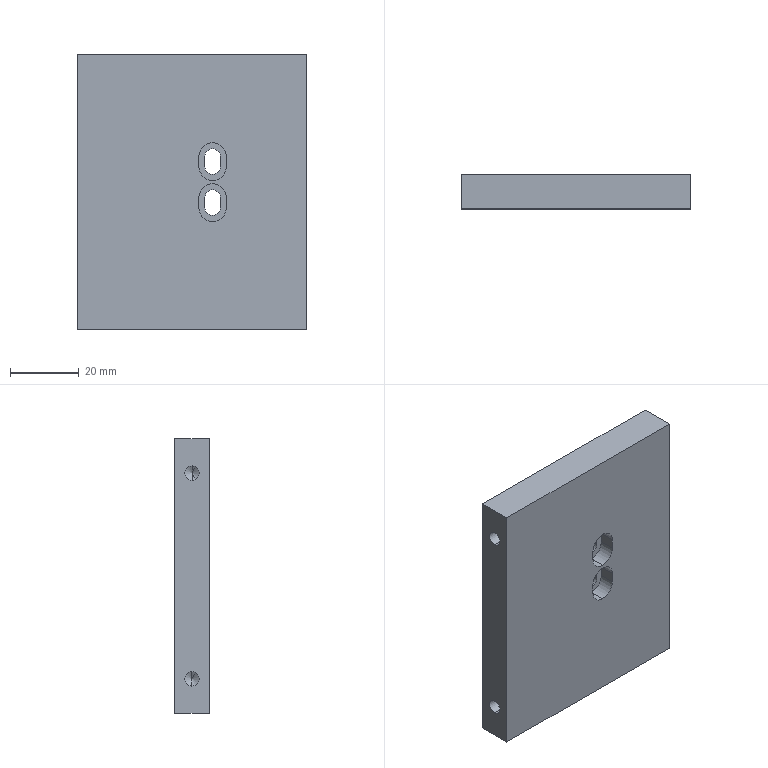Part | SolidWorks | features HoleWzd 2, Extrusion 1, MirrorPattern 1 | 1 solid | 44 faces | box 67 x 10 x 80 mm | volume 51889 mm3 | cylinder 20 | plane 16 | cone 8 | commonest cylinder face diameters 4.2 x8 4.5 x6 8 x6
STEP:
#1=CARTESIAN_POINT('',(6.,-0.4,3.376));
#2=VERTEX_POINT('',#1);
#3=CARTESIAN_POINT('',(10.,-0.4,7.376));
#4=VERTEX_POINT('',#3);
#5=CARTESIAN_POINT('',(6.,-0.4,7.376));
#6=DIRECTION('',(0.,-1.,0.));
#7=DIRECTION('',(0.,0.,-1.));
#8=AXIS2_PLACEMENT_3D('',#5,#6,#7);
#9=CIRCLE('',#8,4.);
#10=EDGE_CURVE('',#2,#4,#9,.T.);
#11=ORIENTED_EDGE('',*,*,#10,.F.);
#12=CARTESIAN_POINT('',(6.,-5.,3.376));
#13=VERTEX_POINT('',#12);
#14=CARTESIAN_POINT('',(6.,-5.,3.376));
#15=DIRECTION('',(0.,-1.,0.));
#16=VECTOR('',#15,1000.);
#17=LINE('',#14,#16);
#18=EDGE_CURVE('',#2,#13,#17,.T.);
#19=ORIENTED_EDGE('',*,*,#18,.T.);
#20=CARTESIAN_POINT('',(10.,-5.,7.376));
#21=VERTEX_POINT('',#20);
#22=CARTESIAN_POINT('',(6.,-5.,7.376));
#23=DIRECTION('',(0.,-1.,0.));
#24=DIRECTION('',(0.,0.,-1.));
#25=AXIS2_PLACEMENT_3D('',#22,#23,#24);
#26=CIRCLE('',#25,4.);
#27=EDGE_CURVE('',#13,#21,#26,.T.);
#28=ORIENTED_EDGE('',*,*,#27,.T.);
#29=CARTESIAN_POINT('',(10.,-0.4,7.376));
#30=DIRECTION('',(0.,1.,0.));
#31=VECTOR('',#30,1000.);
#32=LINE('',#29,#31);
#33=EDGE_CURVE('',#21,#4,#32,.T.);
#34=ORIENTED_EDGE('',*,*,#33,.T.);
#35=EDGE_LOOP('',(#11,#19,#28,#34));
#36=FACE_OUTER_BOUND('',#35,.T.);
#37=CARTESIAN_POINT('',(6.,-5.,7.376));
#38=DIRECTION('',(0.,-1.,0.));
#39=DIRECTION('',(0.,0.,-1.));
#40=AXIS2_PLACEMENT_3D('',#37,#38,#39);
#41=CYLINDRICAL_SURFACE('',#40,4.);
#42=ADVANCED_FACE('',(#36),#41,.F.);
#43=CARTESIAN_POINT('',(6.,5.,5.126));
#44=VERTEX_POINT('',#43);
#45=CARTESIAN_POINT('',(8.25,5.,7.376));
#46=VERTEX_POINT('',#45);
#47=CARTESIAN_POINT('',(6.,5.,7.376));
#48=DIRECTION('',(0.,-1.,0.));
#49=DIRECTION('',(0.,0.,-1.));
#50=AXIS2_PLACEMENT_3D('',#47,#48,#49);
#51=CIRCLE('',#50,2.25);
#52=EDGE_CURVE('',#44,#46,#51,.T.);
#53=ORIENTED_EDGE('',*,*,#52,.F.);
#54=CARTESIAN_POINT('',(6.,-0.4,5.126));
#55=VERTEX_POINT('',#54);
#56=CARTESIAN_POINT('',(6.,-5.,5.126));
#57=DIRECTION('',(0.,-1.,0.));
#58=VECTOR('',#57,1000.);
#59=LINE('',#56,#58);
#60=EDGE_CURVE('',#44,#55,#59,.T.);
#61=ORIENTED_EDGE('',*,*,#60,.T.);
#62=CARTESIAN_POINT('',(8.25,-0.4,7.376));
#63=VERTEX_POINT('',#62);
#64=CARTESIAN_POINT('',(6.,-0.4,7.376));
#65=DIRECTION('',(0.,-1.,0.));
#66=DIRECTION('',(0.,0.,-1.));
#67=AXIS2_PLACEMENT_3D('',#64,#65,#66);
#68=CIRCLE('',#67,2.25);
#69=EDGE_CURVE('',#55,#63,#68,.T.);
#70=ORIENTED_EDGE('',*,*,#69,.T.);
#71=CARTESIAN_POINT('',(8.25,5.,7.376));
#72=DIRECTION('',(0.,1.,0.));
#73=VECTOR('',#72,1000.);
#74=LINE('',#71,#73);
#75=EDGE_CURVE('',#63,#46,#74,.T.);
#76=ORIENTED_EDGE('',*,*,#75,.T.);
#77=EDGE_LOOP('',(#53,#61,#70,#76));
#78=FACE_OUTER_BOUND('',#77,.T.);
#79=CARTESIAN_POINT('',(6.,-5.,7.376));
#80=DIRECTION('',(0.,-1.,0.));
#81=DIRECTION('',(0.,0.,-1.));
#82=AXIS2_PLACEMENT_3D('',#79,#80,#81);
#83=CYLINDRICAL_SURFACE('',#82,2.25);
#84=ADVANCED_FACE('',(#78),#83,.F.);
#85=CARTESIAN_POINT('',(6.,-0.4,-8.624));
#86=VERTEX_POINT('',#85);
#87=CARTESIAN_POINT('',(10.,-0.4,-4.624));
#88=VERTEX_POINT('',#87);
#89=CARTESIAN_POINT('',(6.,-0.4,-4.624));
#90=DIRECTION('',(0.,-1.,0.));
#91=DIRECTION('',(0.,0.,-1.));
#92=AXIS2_PLACEMENT_3D('',#89,#90,#91);
#93=CIRCLE('',#92,4.);
#94=EDGE_CURVE('',#86,#88,#93,.T.);
#95=ORIENTED_EDGE('',*,*,#94,.F.);
#96=CARTESIAN_POINT('',(6.,-5.,-8.624));
#97=VERTEX_POINT('',#96);
#98=CARTESIAN_POINT('',(6.,-5.,-8.624));
#99=DIRECTION('',(0.,-1.,0.));
#100=VECTOR('',#99,1000.);
#101=LINE('',#98,#100);
#102=EDGE_CURVE('',#86,#97,#101,.T.);
#103=ORIENTED_EDGE('',*,*,#102,.T.);
#104=CARTESIAN_POINT('',(10.,-5.,-4.624));
#105=VERTEX_POINT('',#104);
#106=CARTESIAN_POINT('',(6.,-5.,-4.624));
#107=DIRECTION('',(0.,-1.,0.));
#108=DIRECTION('',(0.,0.,-1.));
#109=AXIS2_PLACEMENT_3D('',#106,#107,#108);
#110=CIRCLE('',#109,4.);
#111=EDGE_CURVE('',#97,#105,#110,.T.);
#112=ORIENTED_EDGE('',*,*,#111,.T.);
#113=CARTESIAN_POINT('',(10.,-0.4,-4.624));
#114=DIRECTION('',(0.,1.,0.));
#115=VECTOR('',#114,1000.);
#116=LINE('',#113,#115);
#117=EDGE_CURVE('',#105,#88,#116,.T.);
#118=ORIENTED_EDGE('',*,*,#117,.T.);
#119=EDGE_LOOP('',(#95,#103,#112,#118));
#120=FACE_OUTER_BOUND('',#119,.T.);
#121=CARTESIAN_POINT('',(6.,-5.,-4.624));
#122=DIRECTION('',(0.,-1.,0.));
#123=DIRECTION('',(0.,0.,-1.));
#124=AXIS2_PLACEMENT_3D('',#121,#122,#123);
#125=CYLINDRICAL_SURFACE('',#124,4.);
#126=ADVANCED_FACE('',(#120),#125,.F.);
#127=CARTESIAN_POINT('',(6.,5.,-6.874));
#128=VERTEX_POINT('',#127);
#129=CARTESIAN_POINT('',(8.25,5.,-4.624));
#130=VERTEX_POINT('',#129);
#131=CARTESIAN_POINT('',(6.,5.,-4.624));
#132=DIRECTION('',(0.,-1.,0.));
#133=DIRECTION('',(0.,0.,-1.));
#134=AXIS2_PLACEMENT_3D('',#131,#132,#133);
#135=CIRCLE('',#134,2.25);
#136=EDGE_CURVE('',#128,#130,#135,.T.);
#137=ORIENTED_EDGE('',*,*,#136,.F.);
#138=CARTESIAN_POINT('',(6.,-0.4,-6.874));
#139=VERTEX_POINT('',#138);
#140=CARTESIAN_POINT('',(6.,-5.,-6.874));
#141=DIRECTION('',(0.,-1.,0.));
#142=VECTOR('',#141,1000.);
#143=LINE('',#140,#142);
#144=EDGE_CURVE('',#128,#139,#143,.T.);
#145=ORIENTED_EDGE('',*,*,#144,.T.);
#146=CARTESIAN_POINT('',(8.25,-0.4,-4.624));
#147=VERTEX_POINT('',#146);
#148=CARTESIAN_POINT('',(6.,-0.4,-4.624));
#149=DIRECTION('',(0.,-1.,0.));
#150=DIRECTION('',(0.,0.,-1.));
#151=AXIS2_PLACEMENT_3D('',#148,#149,#150);
#152=CIRCLE('',#151,2.25);
#153=EDGE_CURVE('',#139,#147,#152,.T.);
#154=ORIENTED_EDGE('',*,*,#153,.T.);
#155=CARTESIAN_POINT('',(8.25,5.,-4.624));
#156=DIRECTION('',(0.,1.,0.));
#157=VECTOR('',#156,1000.);
#158=LINE('',#155,#157);
#159=EDGE_CURVE('',#147,#130,#158,.T.);
#160=ORIENTED_EDGE('',*,*,#159,.T.);
#161=EDGE_LOOP('',(#137,#145,#154,#160));
#162=FACE_OUTER_BOUND('',#161,.T.);
#163=CARTESIAN_POINT('',(6.,-5.,-4.624));
#164=DIRECTION('',(0.,-1.,0.));
#165=DIRECTION('',(0.,0.,-1.));
#166=AXIS2_PLACEMENT_3D('',#163,#164,#165);
#167=CYLINDRICAL_SURFACE('',#166,2.25);
#168=ADVANCED_FACE('',(#162),#167,.F.);
#169=CARTESIAN_POINT('',(-21.1,0.,27.9));
#170=VERTEX_POINT('',#169);
#171=CARTESIAN_POINT('',(-21.1,0.,32.1));
#172=VERTEX_POINT('',#171);
#173=CARTESIAN_POINT('',(-21.1,0.,30.));
#174=DIRECTION('',(-1.,0.,0.));
#175=DIRECTION('',(0.,0.,1.));
#176=AXIS2_PLACEMENT_3D('',#173,#174,#175);
#177=CIRCLE('',#176,2.1);
#178=EDGE_CURVE('',#170,#172,#177,.T.);
#179=ORIENTED_EDGE('',*,*,#178,.F.);
#180=CARTESIAN_POINT('',(-33.5,0.,27.9));
#181=VERTEX_POINT('',#180);
#182=CARTESIAN_POINT('',(-33.5,0.,27.9));
#183=DIRECTION('',(-1.,0.,0.));
#184=VECTOR('',#183,1000.);
#185=LINE('',#182,#184);
#186=EDGE_CURVE('',#170,#181,#185,.T.);
#187=ORIENTED_EDGE('',*,*,#186,.T.);
#188=CARTESIAN_POINT('',(-33.5,0.,32.1));
#189=VERTEX_POINT('',#188);
#190=CARTESIAN_POINT('',(-33.5,0.,30.));
#191=DIRECTION('',(-1.,0.,0.));
#192=DIRECTION('',(0.,0.,1.));
#193=AXIS2_PLACEMENT_3D('',#190,#191,#192);
#194=CIRCLE('',#193,2.1);
#195=EDGE_CURVE('',#181,#189,#194,.T.);
#196=ORIENTED_EDGE('',*,*,#195,.T.);
#197=CARTESIAN_POINT('',(-33.5,0.,32.1));
#198=DIRECTION('',(-1.,0.,0.));
#199=VECTOR('',#198,1000.);
#200=LINE('',#197,#199);
#201=EDGE_CURVE('',#172,#189,#200,.T.);
#202=ORIENTED_EDGE('',*,*,#201,.F.);
#203=EDGE_LOOP('',(#179,#187,#196,#202));
#204=FACE_OUTER_BOUND('',#203,.T.);
#205=CARTESIAN_POINT('',(-33.5,0.,30.));
#206=DIRECTION('',(-1.,0.,0.));
#207=DIRECTION('',(0.,0.,1.));
#208=AXIS2_PLACEMENT_3D('',#205,#206,#207);
#209=CYLINDRICAL_SURFACE('',#208,2.1);
#210=ADVANCED_FACE('',(#204),#209,.F.);
#211=CARTESIAN_POINT('',(-19.838,0.,30.));
#212=VERTEX_POINT('',#211);
#213=CARTESIAN_POINT('',(-21.1,0.,32.1));
#214=DIRECTION('',(-0.515,0.,0.8572));
#215=VECTOR('',#214,1000.);
#216=LINE('',#213,#215);
#217=EDGE_CURVE('',#212,#172,#216,.T.);
#218=ORIENTED_EDGE('',*,*,#217,.F.);
#219=CARTESIAN_POINT('',(-21.1,0.,27.9));
#220=DIRECTION('',(-0.515,0.,-0.8572));
#221=VECTOR('',#220,1000.);
#222=LINE('',#219,#221);
#223=EDGE_CURVE('',#212,#170,#222,.T.);
#224=ORIENTED_EDGE('',*,*,#223,.T.);
#225=ORIENTED_EDGE('',*,*,#178,.T.);
#226=EDGE_LOOP('',(#218,#224,#225));
#227=FACE_OUTER_BOUND('',#226,.T.);
#228=CARTESIAN_POINT('',(-21.1,0.,30.));
#229=DIRECTION('',(-1.,0.,0.));
#230=DIRECTION('',(0.,0.,1.));
#231=AXIS2_PLACEMENT_3D('',#228,#229,#230);
#232=CONICAL_SURFACE('',#231,2.1,1.03);
#233=ADVANCED_FACE('',(#227),#232,.F.);
#234=CARTESIAN_POINT('',(-21.1,0.,-32.1));
#235=VERTEX_POINT('',#234);
#236=CARTESIAN_POINT('',(-21.1,0.,-27.9));
#237=VERTEX_POINT('',#236);
#238=CARTESIAN_POINT('',(-21.1,0.,-30.));
#239=DIRECTION('',(-1.,0.,0.));
#240=DIRECTION('',(0.,0.,1.));
#241=AXIS2_PLACEMENT_3D('',#238,#239,#240);
#242=CIRCLE('',#241,2.1);
#243=EDGE_CURVE('',#235,#237,#242,.T.);
#244=ORIENTED_EDGE('',*,*,#243,.F.);
#245=CARTESIAN_POINT('',(-33.5,0.,-32.1));
#246=VERTEX_POINT('',#245);
#247=CARTESIAN_POINT('',(-33.5,0.,-32.1));
#248=DIRECTION('',(-1.,0.,0.));
#249=VECTOR('',#248,1000.);
#250=LINE('',#247,#249);
#251=EDGE_CURVE('',#235,#246,#250,.T.);
#252=ORIENTED_EDGE('',*,*,#251,.T.);
#253=CARTESIAN_POINT('',(-33.5,0.,-27.9));
#254=VERTEX_POINT('',#253);
#255=CARTESIAN_POINT('',(-33.5,0.,-30.));
#256=DIRECTION('',(-1.,0.,0.));
#257=DIRECTION('',(0.,0.,1.));
#258=AXIS2_PLACEMENT_3D('',#255,#256,#257);
#259=CIRCLE('',#258,2.1);
#260=EDGE_CURVE('',#246,#254,#259,.T.);
#261=ORIENTED_EDGE('',*,*,#260,.T.);
#262=CARTESIAN_POINT('',(-33.5,0.,-27.9));
#263=DIRECTION('',(-1.,0.,0.));
#264=VECTOR('',#263,1000.);
#265=LINE('',#262,#264);
#266=EDGE_CURVE('',#237,#254,#265,.T.);
#267=ORIENTED_EDGE('',*,*,#266,.F.);
#268=EDGE_LOOP('',(#244,#252,#261,#267));
#269=FACE_OUTER_BOUND('',#268,.T.);
#270=CARTESIAN_POINT('',(-33.5,0.,-30.));
#271=DIRECTION('',(-1.,0.,0.));
#272=DIRECTION('',(0.,0.,1.));
#273=AXIS2_PLACEMENT_3D('',#270,#271,#272);
#274=CYLINDRICAL_SURFACE('',#273,2.1);
#275=ADVANCED_FACE('',(#269),#274,.F.);
#276=CARTESIAN_POINT('',(-19.838,0.,-30.));
#277=VERTEX_POINT('',#276);
#278=CARTESIAN_POINT('',(-21.1,0.,-27.9));
#279=DIRECTION('',(-0.515,0.,0.8572));
#280=VECTOR('',#279,1000.);
#281=LINE('',#278,#280);
#282=EDGE_CURVE('',#277,#237,#281,.T.);
#283=ORIENTED_EDGE('',*,*,#282,.F.);
#284=CARTESIAN_POINT('',(-21.1,0.,-32.1));
#285=DIRECTION('',(-0.515,0.,-0.8572));
#286=VECTOR('',#285,1000.);
#287=LINE('',#284,#286);
#288=EDGE_CURVE('',#277,#235,#287,.T.);
#289=ORIENTED_EDGE('',*,*,#288,.T.);
#290=ORIENTED_EDGE('',*,*,#243,.T.);
#291=EDGE_LOOP('',(#283,#289,#290));
#292=FACE_OUTER_BOUND('',#291,.T.);
#293=CARTESIAN_POINT('',(-21.1,0.,-30.));
#294=DIRECTION('',(-1.,0.,0.));
#295=DIRECTION('',(0.,0.,1.));
#296=AXIS2_PLACEMENT_3D('',#293,#294,#295);
#297=CONICAL_SURFACE('',#296,2.1,1.03);
#298=ADVANCED_FACE('',(#292),#297,.F.);
#299=CARTESIAN_POINT('',(21.1,0.,32.1));
#300=VERTEX_POINT('',#299);
#301=CARTESIAN_POINT('',(21.1,0.,27.9));
#302=VERTEX_POINT('',#301);
#303=CARTESIAN_POINT('',(21.1,0.,30.));
#304=DIRECTION('',(1.,0.,0.));
#305=DIRECTION('',(0.,0.,-1.));
#306=AXIS2_PLACEMENT_3D('',#303,#304,#305);
#307=CIRCLE('',#306,2.1);
#308=EDGE_CURVE('',#300,#302,#307,.T.);
#309=ORIENTED_EDGE('',*,*,#308,.F.);
#310=CARTESIAN_POINT('',(33.5,0.,32.1));
#311=VERTEX_POINT('',#310);
#312=CARTESIAN_POINT('',(33.5,0.,32.1));
#313=DIRECTION('',(1.,0.,0.));
#314=VECTOR('',#313,1000.);
#315=LINE('',#312,#314);
#316=EDGE_CURVE('',#300,#311,#315,.T.);
#317=ORIENTED_EDGE('',*,*,#316,.T.);
#318=CARTESIAN_POINT('',(33.5,0.,27.9));
#319=VERTEX_POINT('',#318);
#320=CARTESIAN_POINT('',(33.5,0.,30.));
#321=DIRECTION('',(1.,0.,0.));
#322=DIRECTION('',(0.,0.,-1.));
#323=AXIS2_PLACEMENT_3D('',#320,#321,#322);
#324=CIRCLE('',#323,2.1);
#325=EDGE_CURVE('',#311,#319,#324,.T.);
#326=ORIENTED_EDGE('',*,*,#325,.T.);
#327=CARTESIAN_POINT('',(33.5,0.,27.9));
#328=DIRECTION('',(1.,0.,0.));
#329=VECTOR('',#328,1000.);
#330=LINE('',#327,#329);
#331=EDGE_CURVE('',#302,#319,#330,.T.);
#332=ORIENTED_EDGE('',*,*,#331,.F.);
#333=EDGE_LOOP('',(#309,#317,#326,#332));
#334=FACE_OUTER_BOUND('',#333,.T.);
#335=CARTESIAN_POINT('',(33.5,0.,30.));
#336=DIRECTION('',(1.,0.,0.));
#337=DIRECTION('',(0.,0.,-1.));
#338=AXIS2_PLACEMENT_3D('',#335,#336,#337);
#339=CYLINDRICAL_SURFACE('',#338,2.1);
#340=ADVANCED_FACE('',(#334),#339,.F.);
#341=CARTESIAN_POINT('',(19.838,0.,30.));
#342=VERTEX_POINT('',#341);
#343=CARTESIAN_POINT('',(21.1,0.,27.9));
#344=DIRECTION('',(0.515,0.,-0.8572));
#345=VECTOR('',#344,1000.);
#346=LINE('',#343,#345);
#347=EDGE_CURVE('',#342,#302,#346,.T.);
#348=ORIENTED_EDGE('',*,*,#347,.F.);
#349=CARTESIAN_POINT('',(21.1,0.,32.1));
#350=DIRECTION('',(0.515,0.,0.8572));
#351=VECTOR('',#350,1000.);
#352=LINE('',#349,#351);
#353=EDGE_CURVE('',#342,#300,#352,.T.);
#354=ORIENTED_EDGE('',*,*,#353,.T.);
#355=ORIENTED_EDGE('',*,*,#308,.T.);
#356=EDGE_LOOP('',(#348,#354,#355));
#357=FACE_OUTER_BOUND('',#356,.T.);
#358=CARTESIAN_POINT('',(21.1,0.,30.));
#359=DIRECTION('',(1.,0.,0.));
#360=DIRECTION('',(0.,0.,-1.));
#361=AXIS2_PLACEMENT_3D('',#358,#359,#360);
#362=CONICAL_SURFACE('',#361,2.1,1.03);
#363=ADVANCED_FACE('',(#357),#362,.F.);
#364=CARTESIAN_POINT('',(21.1,0.,-27.9));
#365=VERTEX_POINT('',#364);
#366=CARTESIAN_POINT('',(21.1,0.,-32.1));
#367=VERTEX_POINT('',#366);
#368=CARTESIAN_POINT('',(21.1,0.,-30.));
#369=DIRECTION('',(1.,0.,0.));
#370=DIRECTION('',(0.,0.,-1.));
#371=AXIS2_PLACEMENT_3D('',#368,#369,#370);
#372=CIRCLE('',#371,2.1);
#373=EDGE_CURVE('',#365,#367,#372,.T.);
#374=ORIENTED_EDGE('',*,*,#373,.F.);
#375=CARTESIAN_POINT('',(33.5,0.,-27.9));
#376=VERTEX_POINT('',#375);
#377=CARTESIAN_POINT('',(33.5,0.,-27.9));
#378=DIRECTION('',(1.,0.,0.));
#379=VECTOR('',#378,1000.);
#380=LINE('',#377,#379);
#381=EDGE_CURVE('',#365,#376,#380,.T.);
#382=ORIENTED_EDGE('',*,*,#381,.T.);
#383=CARTESIAN_POINT('',(33.5,0.,-32.1));
#384=VERTEX_POINT('',#383);
#385=CARTESIAN_POINT('',(33.5,0.,-30.));
#386=DIRECTION('',(1.,0.,0.));
#387=DIRECTION('',(0.,0.,-1.));
#388=AXIS2_PLACEMENT_3D('',#385,#386,#387);
#389=CIRCLE('',#388,2.1);
#390=EDGE_CURVE('',#376,#384,#389,.T.);
#391=ORIENTED_EDGE('',*,*,#390,.T.);
#392=CARTESIAN_POINT('',(33.5,0.,-32.1));
#393=DIRECTION('',(1.,0.,0.));
#394=VECTOR('',#393,1000.);
#395=LINE('',#392,#394);
#396=EDGE_CURVE('',#367,#384,#395,.T.);
#397=ORIENTED_EDGE('',*,*,#396,.F.);
#398=EDGE_LOOP('',(#374,#382,#391,#397));
#399=FACE_OUTER_BOUND('',#398,.T.);
#400=CARTESIAN_POINT('',(33.5,0.,-30.));
#401=DIRECTION('',(1.,0.,0.));
#402=DIRECTION('',(0.,0.,-1.));
#403=AXIS2_PLACEMENT_3D('',#400,#401,#402);
#404=CYLINDRICAL_SURFACE('',#403,2.1);
#405=ADVANCED_FACE('',(#399),#404,.F.);
#406=CARTESIAN_POINT('',(19.838,0.,-30.));
#407=VERTEX_POINT('',#406);
#408=CARTESIAN_POINT('',(21.1,0.,-32.1));
#409=DIRECTION('',(0.515,0.,-0.8572));
#410=VECTOR('',#409,1000.);
#411=LINE('',#408,#410);
#412=EDGE_CURVE('',#407,#367,#411,.T.);
#413=ORIENTED_EDGE('',*,*,#412,.F.);
#414=CARTESIAN_POINT('',(21.1,0.,-27.9));
#415=DIRECTION('',(0.515,0.,0.8572));
#416=VECTOR('',#415,1000.);
#417=LINE('',#414,#416);
#418=EDGE_CURVE('',#407,#365,#417,.T.);
#419=ORIENTED_EDGE('',*,*,#418,.T.);
#420=ORIENTED_EDGE('',*,*,#373,.T.);
#421=EDGE_LOOP('',(#413,#419,#420));
#422=FACE_OUTER_BOUND('',#421,.T.);
#423=CARTESIAN_POINT('',(21.1,0.,-30.));
#424=DIRECTION('',(1.,0.,0.));
#425=DIRECTION('',(0.,0.,-1.));
#426=AXIS2_PLACEMENT_3D('',#423,#424,#425);
#427=CONICAL_SURFACE('',#426,2.1,1.03);
#428=ADVANCED_FACE('',(#422),#427,.F.);
#429=CARTESIAN_POINT('',(-33.5,-5.,-40.));
#430=VERTEX_POINT('',#429);
#431=CARTESIAN_POINT('',(-33.5,5.,-40.));
#432=VERTEX_POINT('',#431);
#433=CARTESIAN_POINT('',(-33.5,5.,-40.));
#434=DIRECTION('',(0.,1.,0.));
#435=VECTOR('',#434,1000.);
#436=LINE('',#433,#435);
#437=EDGE_CURVE('',#430,#432,#436,.T.);
#438=ORIENTED_EDGE('',*,*,#437,.T.);
#439=CARTESIAN_POINT('',(33.5,5.,-40.));
#440=VERTEX_POINT('',#439);
#441=CARTESIAN_POINT('',(33.5,5.,-40.));
#442=DIRECTION('',(-1.,0.,0.));
#443=VECTOR('',#442,1000.);
#444=LINE('',#441,#443);
#445=EDGE_CURVE('',#440,#432,#444,.T.);
#446=ORIENTED_EDGE('',*,*,#445,.F.);
#447=CARTESIAN_POINT('',(33.5,-5.,-40.));
#448=VERTEX_POINT('',#447);
#449=CARTESIAN_POINT('',(33.5,5.,-40.));
#450=DIRECTION('',(0.,1.,0.));
#451=VECTOR('',#450,1000.);
#452=LINE('',#449,#451);
#453=EDGE_CURVE('',#448,#440,#452,.T.);
#454=ORIENTED_EDGE('',*,*,#453,.F.);
#455=CARTESIAN_POINT('',(33.5,-5.,-40.));
#456=DIRECTION('',(-1.,0.,0.));
#457=VECTOR('',#456,1000.);
#458=LINE('',#455,#457);
#459=EDGE_CURVE('',#448,#430,#458,.T.);
#460=ORIENTED_EDGE('',*,*,#459,.T.);
#461=EDGE_LOOP('',(#438,#446,#454,#460));
#462=FACE_OUTER_BOUND('',#461,.T.);
#463=CARTESIAN_POINT('',(33.5,5.,-40.));
#464=DIRECTION('',(0.,0.,1.));
#465=DIRECTION('',(1.,0.,0.));
#466=AXIS2_PLACEMENT_3D('',#463,#464,#465);
#467=PLANE('',#466);
#468=ADVANCED_FACE('',(#462),#467,.F.);
#469=CARTESIAN_POINT('',(3.75,5.,10.376));
#470=VERTEX_POINT('',#469);
#471=CARTESIAN_POINT('',(3.75,5.,7.376));
#472=VERTEX_POINT('',#471);
#473=CARTESIAN_POINT('',(3.75,5.,10.376));
#474=DIRECTION('',(0.,0.,-1.));
#475=VECTOR('',#474,1000.);
#476=LINE('',#473,#475);
#477=EDGE_CURVE('',#470,#472,#476,.T.);
#478=ORIENTED_EDGE('',*,*,#477,.T.);
#479=CARTESIAN_POINT('',(6.,5.,7.376));
#480=DIRECTION('',(0.,-1.,0.));
#481=DIRECTION('',(0.,0.,-1.));
#482=AXIS2_PLACEMENT_3D('',#479,#480,#481);
#483=CIRCLE('',#482,2.25);
#484=EDGE_CURVE('',#472,#44,#483,.T.);
#485=ORIENTED_EDGE('',*,*,#484,.T.);
#486=ORIENTED_EDGE('',*,*,#52,.T.);
#487=CARTESIAN_POINT('',(8.25,5.,10.376));
#488=VERTEX_POINT('',#487);
#489=CARTESIAN_POINT('',(8.25,5.,10.376));
#490=DIRECTION('',(0.,0.,-1.));
#491=VECTOR('',#490,1000.);
#492=LINE('',#489,#491);
#493=EDGE_CURVE('',#488,#46,#492,.T.);
#494=ORIENTED_EDGE('',*,*,#493,.F.);
#495=CARTESIAN_POINT('',(6.,5.,10.376));
#496=DIRECTION('',(0.,-1.,0.));
#497=DIRECTION('',(0.,0.,-1.));
#498=AXIS2_PLACEMENT_3D('',#495,#496,#497);
#499=CIRCLE('',#498,2.25);
#500=EDGE_CURVE('',#488,#470,#499,.T.);
#501=ORIENTED_EDGE('',*,*,#500,.T.);
#502=EDGE_LOOP('',(#478,#485,#486,#494,#501));
#503=FACE_BOUND('',#502,.T.);
#504=CARTESIAN_POINT('',(3.75,5.,-1.624));
#505=VERTEX_POINT('',#504);
#506=CARTESIAN_POINT('',(3.75,5.,-4.624));
#507=VERTEX_POINT('',#506);
#508=CARTESIAN_POINT('',(3.75,5.,-1.624));
#509=DIRECTION('',(0.,0.,-1.));
#510=VECTOR('',#509,1000.);
#511=LINE('',#508,#510);
#512=EDGE_CURVE('',#505,#507,#511,.T.);
#513=ORIENTED_EDGE('',*,*,#512,.T.);
#514=CARTESIAN_POINT('',(6.,5.,-4.624));
#515=DIRECTION('',(0.,-1.,0.));
#516=DIRECTION('',(0.,0.,-1.));
#517=AXIS2_PLACEMENT_3D('',#514,#515,#516);
#518=CIRCLE('',#517,2.25);
#519=EDGE_CURVE('',#507,#128,#518,.T.);
#520=ORIENTED_EDGE('',*,*,#519,.T.);
#521=ORIENTED_EDGE('',*,*,#136,.T.);
#522=CARTESIAN_POINT('',(8.25,5.,-1.624));
#523=VERTEX_POINT('',#522);
#524=CARTESIAN_POINT('',(8.25,5.,-1.624));
#525=DIRECTION('',(0.,0.,-1.));
#526=VECTOR('',#525,1000.);
#527=LINE('',#524,#526);
#528=EDGE_CURVE('',#523,#130,#527,.T.);
#529=ORIENTED_EDGE('',*,*,#528,.F.);
#530=CARTESIAN_POINT('',(6.,5.,-1.624));
#531=DIRECTION('',(0.,-1.,0.));
#532=DIRECTION('',(0.,0.,-1.));
#533=AXIS2_PLACEMENT_3D('',#530,#531,#532);
#534=CIRCLE('',#533,2.25);
#535=EDGE_CURVE('',#523,#505,#534,.T.);
#536=ORIENTED_EDGE('',*,*,#535,.T.);
#537=EDGE_LOOP('',(#513,#520,#521,#529,#536));
#538=FACE_BOUND('',#537,.T.);
#539=CARTESIAN_POINT('',(-33.5,5.,40.));
#540=VERTEX_POINT('',#539);
#541=CARTESIAN_POINT('',(-33.5,5.,40.));
#542=DIRECTION('',(0.,0.,1.));
#543=VECTOR('',#542,1000.);
#544=LINE('',#541,#543);
#545=EDGE_CURVE('',#432,#540,#544,.T.);
#546=ORIENTED_EDGE('',*,*,#545,.T.);
#547=CARTESIAN_POINT('',(33.5,5.,40.));
#548=VERTEX_POINT('',#547);
#549=CARTESIAN_POINT('',(33.5,5.,40.));
#550=DIRECTION('',(-1.,0.,0.));
#551=VECTOR('',#550,1000.);
#552=LINE('',#549,#551);
#553=EDGE_CURVE('',#548,#540,#552,.T.);
#554=ORIENTED_EDGE('',*,*,#553,.F.);
#555=CARTESIAN_POINT('',(33.5,5.,40.));
#556=DIRECTION('',(0.,0.,1.));
#557=VECTOR('',#556,1000.);
#558=LINE('',#555,#557);
#559=EDGE_CURVE('',#440,#548,#558,.T.);
#560=ORIENTED_EDGE('',*,*,#559,.F.);
#561=ORIENTED_EDGE('',*,*,#445,.T.);
#562=EDGE_LOOP('',(#546,#554,#560,#561));
#563=FACE_OUTER_BOUND('',#562,.T.);
#564=CARTESIAN_POINT('',(33.5,5.,40.));
#565=DIRECTION('',(0.,-1.,0.));
#566=DIRECTION('',(0.,0.,-1.));
#567=AXIS2_PLACEMENT_3D('',#564,#565,#566);
#568=PLANE('',#567);
#569=ADVANCED_FACE('',(#503,#538,#563),#568,.F.);
#570=CARTESIAN_POINT('',(-33.5,-5.,40.));
#571=VERTEX_POINT('',#570);
#572=CARTESIAN_POINT('',(-33.5,5.,40.));
#573=DIRECTION('',(0.,-1.,0.));
#574=VECTOR('',#573,1000.);
#575=LINE('',#572,#574);
#576=EDGE_CURVE('',#540,#571,#575,.T.);
#577=ORIENTED_EDGE('',*,*,#576,.T.);
#578=CARTESIAN_POINT('',(33.5,-5.,40.));
#579=VERTEX_POINT('',#578);
#580=CARTESIAN_POINT('',(33.5,-5.,40.));
#581=DIRECTION('',(-1.,0.,0.));
#582=VECTOR('',#581,1000.);
#583=LINE('',#580,#582);
#584=EDGE_CURVE('',#579,#571,#583,.T.);
#585=ORIENTED_EDGE('',*,*,#584,.F.);
#586=CARTESIAN_POINT('',(33.5,5.,40.));
#587=DIRECTION('',(0.,-1.,0.));
#588=VECTOR('',#587,1000.);
#589=LINE('',#586,#588);
#590=EDGE_CURVE('',#548,#579,#589,.T.);
#591=ORIENTED_EDGE('',*,*,#590,.F.);
#592=ORIENTED_EDGE('',*,*,#553,.T.);
#593=EDGE_LOOP('',(#577,#585,#591,#592));
#594=FACE_OUTER_BOUND('',#593,.T.);
#595=CARTESIAN_POINT('',(33.5,5.,40.));
#596=DIRECTION('',(0.,0.,-1.));
#597=DIRECTION('',(-1.,0.,0.));
#598=AXIS2_PLACEMENT_3D('',#595,#596,#597);
#599=PLANE('',#598);
#600=ADVANCED_FACE('',(#594),#599,.F.);
#601=CARTESIAN_POINT('',(10.,-5.,10.376));
#602=VERTEX_POINT('',#601);
#603=CARTESIAN_POINT('',(10.,-5.,10.376));
#604=DIRECTION('',(0.,0.,-1.));
#605=VECTOR('',#604,1000.);
#606=LINE('',#603,#605);
#607=EDGE_CURVE('',#602,#21,#606,.T.);
#608=ORIENTED_EDGE('',*,*,#607,.T.);
#609=ORIENTED_EDGE('',*,*,#27,.F.);
#610=CARTESIAN_POINT('',(2.,-5.,7.376));
#611=VERTEX_POINT('',#610);
#612=CARTESIAN_POINT('',(6.,-5.,7.376));
#613=DIRECTION('',(0.,-1.,0.));
#614=DIRECTION('',(0.,0.,-1.));
#615=AXIS2_PLACEMENT_3D('',#612,#613,#614);
#616=CIRCLE('',#615,4.);
#617=EDGE_CURVE('',#611,#13,#616,.T.);
#618=ORIENTED_EDGE('',*,*,#617,.F.);
#619=CARTESIAN_POINT('',(2.,-5.,10.376));
#620=VERTEX_POINT('',#619);
#621=CARTESIAN_POINT('',(2.,-5.,10.376));
#622=DIRECTION('',(0.,0.,-1.));
#623=VECTOR('',#622,1000.);
#624=LINE('',#621,#623);
#625=EDGE_CURVE('',#620,#611,#624,.T.);
#626=ORIENTED_EDGE('',*,*,#625,.F.);
#627=CARTESIAN_POINT('',(6.,-5.,10.376));
#628=DIRECTION('',(0.,-1.,0.));
#629=DIRECTION('',(0.,0.,-1.));
#630=AXIS2_PLACEMENT_3D('',#627,#628,#629);
#631=CIRCLE('',#630,4.);
#632=EDGE_CURVE('',#602,#620,#631,.T.);
#633=ORIENTED_EDGE('',*,*,#632,.F.);
#634=EDGE_LOOP('',(#608,#609,#618,#626,#633));
#635=FACE_BOUND('',#634,.T.);
#636=CARTESIAN_POINT('',(2.,-5.,-4.624));
#637=VERTEX_POINT('',#636);
#638=CARTESIAN_POINT('',(6.,-5.,-4.624));
#639=DIRECTION('',(0.,-1.,0.));
#640=DIRECTION('',(0.,0.,-1.));
#641=AXIS2_PLACEMENT_3D('',#638,#639,#640);
#642=CIRCLE('',#641,4.);
#643=EDGE_CURVE('',#637,#97,#642,.T.);
#644=ORIENTED_EDGE('',*,*,#643,.F.);
#645=CARTESIAN_POINT('',(2.,-5.,-1.624));
#646=VERTEX_POINT('',#645);
#647=CARTESIAN_POINT('',(2.,-5.,-1.624));
#648=DIRECTION('',(0.,0.,-1.));
#649=VECTOR('',#648,1000.);
#650=LINE('',#647,#649);
#651=EDGE_CURVE('',#646,#637,#650,.T.);
#652=ORIENTED_EDGE('',*,*,#651,.F.);
#653=CARTESIAN_POINT('',(10.,-5.,-1.624));
#654=VERTEX_POINT('',#653);
#655=CARTESIAN_POINT('',(6.,-5.,-1.624));
#656=DIRECTION('',(0.,-1.,0.));
#657=DIRECTION('',(0.,0.,-1.));
#658=AXIS2_PLACEMENT_3D('',#655,#656,#657);
#659=CIRCLE('',#658,4.);
#660=EDGE_CURVE('',#654,#646,#659,.T.);
#661=ORIENTED_EDGE('',*,*,#660,.F.);
#662=CARTESIAN_POINT('',(10.,-5.,-1.624));
#663=DIRECTION('',(0.,0.,-1.));
#664=VECTOR('',#663,1000.);
#665=LINE('',#662,#664);
#666=EDGE_CURVE('',#654,#105,#665,.T.);
#667=ORIENTED_EDGE('',*,*,#666,.T.);
#668=ORIENTED_EDGE('',*,*,#111,.F.);
#669=EDGE_LOOP('',(#644,#652,#661,#667,#668));
#670=FACE_BOUND('',#669,.T.);
#671=CARTESIAN_POINT('',(-33.5,-5.,40.));
#672=DIRECTION('',(0.,0.,-1.));
#673=VECTOR('',#672,1000.);
#674=LINE('',#671,#673);
#675=EDGE_CURVE('',#571,#430,#674,.T.);
#676=ORIENTED_EDGE('',*,*,#675,.T.);
#677=ORIENTED_EDGE('',*,*,#459,.F.);
#678=CARTESIAN_POINT('',(33.5,-5.,40.));
#679=DIRECTION('',(0.,0.,-1.));
#680=VECTOR('',#679,1000.);
#681=LINE('',#678,#680);
#682=EDGE_CURVE('',#579,#448,#681,.T.);
#683=ORIENTED_EDGE('',*,*,#682,.F.);
#684=ORIENTED_EDGE('',*,*,#584,.T.);
#685=EDGE_LOOP('',(#676,#677,#683,#684));
#686=FACE_OUTER_BOUND('',#685,.T.);
#687=CARTESIAN_POINT('',(33.5,-5.,40.));
#688=DIRECTION('',(0.,1.,0.));
#689=DIRECTION('',(0.,0.,1.));
#690=AXIS2_PLACEMENT_3D('',#687,#688,#689);
#691=PLANE('',#690);
#692=ADVANCED_FACE('',(#635,#670,#686),#691,.F.);
#693=CARTESIAN_POINT('',(33.5,0.,30.));
#694=DIRECTION('',(1.,0.,0.));
#695=DIRECTION('',(0.,0.,-1.));
#696=AXIS2_PLACEMENT_3D('',#693,#694,#695);
#697=CIRCLE('',#696,2.1);
#698=EDGE_CURVE('',#319,#311,#697,.T.);
#699=ORIENTED_EDGE('',*,*,#698,.F.);
#700=ORIENTED_EDGE('',*,*,#325,.F.);
#701=EDGE_LOOP('',(#699,#700));
#702=FACE_BOUND('',#701,.T.);
#703=CARTESIAN_POINT('',(33.5,0.,-30.));
#704=DIRECTION('',(1.,0.,0.));
#705=DIRECTION('',(0.,0.,-1.));
#706=AXIS2_PLACEMENT_3D('',#703,#704,#705);
#707=CIRCLE('',#706,2.1);
#708=EDGE_CURVE('',#384,#376,#707,.T.);
#709=ORIENTED_EDGE('',*,*,#708,.F.);
#710=ORIENTED_EDGE('',*,*,#390,.F.);
#711=EDGE_LOOP('',(#709,#710));
#712=FACE_BOUND('',#711,.T.);
#713=ORIENTED_EDGE('',*,*,#453,.T.);
#714=ORIENTED_EDGE('',*,*,#559,.T.);
#715=ORIENTED_EDGE('',*,*,#590,.T.);
#716=ORIENTED_EDGE('',*,*,#682,.T.);
#717=EDGE_LOOP('',(#713,#714,#715,#716));
#718=FACE_OUTER_BOUND('',#717,.T.);
#719=CARTESIAN_POINT('',(33.5,0.,0.));
#720=DIRECTION('',(1.,0.,0.));
#721=DIRECTION('',(0.,0.,-1.));
#722=AXIS2_PLACEMENT_3D('',#719,#720,#721);
#723=PLANE('',#722);
#724=ADVANCED_FACE('',(#702,#712,#718),#723,.T.);
#725=CARTESIAN_POINT('',(-33.5,0.,30.));
#726=DIRECTION('',(-1.,0.,0.));
#727=DIRECTION('',(0.,0.,1.));
#728=AXIS2_PLACEMENT_3D('',#725,#726,#727);
#729=CIRCLE('',#728,2.1);
#730=EDGE_CURVE('',#189,#181,#729,.T.);
#731=ORIENTED_EDGE('',*,*,#730,.F.);
#732=ORIENTED_EDGE('',*,*,#195,.F.);
#733=EDGE_LOOP('',(#731,#732));
#734=FACE_BOUND('',#733,.T.);
#735=CARTESIAN_POINT('',(-33.5,0.,-30.));
#736=DIRECTION('',(-1.,0.,0.));
#737=DIRECTION('',(0.,0.,1.));
#738=AXIS2_PLACEMENT_3D('',#735,#736,#737);
#739=CIRCLE('',#738,2.1);
#740=EDGE_CURVE('',#254,#246,#739,.T.);
#741=ORIENTED_EDGE('',*,*,#740,.F.);
#742=ORIENTED_EDGE('',*,*,#260,.F.);
#743=EDGE_LOOP('',(#741,#742));
#744=FACE_BOUND('',#743,.T.);
#745=ORIENTED_EDGE('',*,*,#437,.F.);
#746=ORIENTED_EDGE('',*,*,#675,.F.);
#747=ORIENTED_EDGE('',*,*,#576,.F.);
#748=ORIENTED_EDGE('',*,*,#545,.F.);
#749=EDGE_LOOP('',(#745,#746,#747,#748));
#750=FACE_OUTER_BOUND('',#749,.T.);
#751=CARTESIAN_POINT('',(-33.5,0.,0.));
#752=DIRECTION('',(1.,0.,0.));
#753=DIRECTION('',(0.,0.,-1.));
#754=AXIS2_PLACEMENT_3D('',#751,#752,#753);
#755=PLANE('',#754);
#756=ADVANCED_FACE('',(#734,#744,#750),#755,.F.);
#757=ORIENTED_EDGE('',*,*,#418,.F.);
#758=ORIENTED_EDGE('',*,*,#412,.T.);
#759=CARTESIAN_POINT('',(21.1,0.,-30.));
#760=DIRECTION('',(1.,0.,0.));
#761=DIRECTION('',(0.,0.,-1.));
#762=AXIS2_PLACEMENT_3D('',#759,#760,#761);
#763=CIRCLE('',#762,2.1);
#764=EDGE_CURVE('',#367,#365,#763,.T.);
#765=ORIENTED_EDGE('',*,*,#764,.T.);
#766=EDGE_LOOP('',(#757,#758,#765));
#767=FACE_OUTER_BOUND('',#766,.T.);
#768=CARTESIAN_POINT('',(21.1,0.,-30.));
#769=DIRECTION('',(1.,0.,0.));
#770=DIRECTION('',(0.,0.,-1.));
#771=AXIS2_PLACEMENT_3D('',#768,#769,#770);
#772=CONICAL_SURFACE('',#771,2.1,1.03);
#773=ADVANCED_FACE('',(#767),#772,.F.);
#774=ORIENTED_EDGE('',*,*,#381,.F.);
#775=ORIENTED_EDGE('',*,*,#764,.F.);
#776=ORIENTED_EDGE('',*,*,#396,.T.);
#777=ORIENTED_EDGE('',*,*,#708,.T.);
#778=EDGE_LOOP('',(#774,#775,#776,#777));
#779=FACE_OUTER_BOUND('',#778,.T.);
#780=CARTESIAN_POINT('',(33.5,0.,-30.));
#781=DIRECTION('',(1.,0.,0.));
#782=DIRECTION('',(0.,0.,-1.));
#783=AXIS2_PLACEMENT_3D('',#780,#781,#782);
#784=CYLINDRICAL_SURFACE('',#783,2.1);
#785=ADVANCED_FACE('',(#779),#784,.F.);
#786=ORIENTED_EDGE('',*,*,#353,.F.);
#787=ORIENTED_EDGE('',*,*,#347,.T.);
#788=CARTESIAN_POINT('',(21.1,0.,30.));
#789=DIRECTION('',(1.,0.,0.));
#790=DIRECTION('',(0.,0.,-1.));
#791=AXIS2_PLACEMENT_3D('',#788,#789,#790);
#792=CIRCLE('',#791,2.1);
#793=EDGE_CURVE('',#302,#300,#792,.T.);
#794=ORIENTED_EDGE('',*,*,#793,.T.);
#795=EDGE_LOOP('',(#786,#787,#794));
#796=FACE_OUTER_BOUND('',#795,.T.);
#797=CARTESIAN_POINT('',(21.1,0.,30.));
#798=DIRECTION('',(1.,0.,0.));
#799=DIRECTION('',(0.,0.,-1.));
#800=AXIS2_PLACEMENT_3D('',#797,#798,#799);
#801=CONICAL_SURFACE('',#800,2.1,1.03);
#802=ADVANCED_FACE('',(#796),#801,.F.);
#803=ORIENTED_EDGE('',*,*,#316,.F.);
#804=ORIENTED_EDGE('',*,*,#793,.F.);
#805=ORIENTED_EDGE('',*,*,#331,.T.);
#806=ORIENTED_EDGE('',*,*,#698,.T.);
#807=EDGE_LOOP('',(#803,#804,#805,#806));
#808=FACE_OUTER_BOUND('',#807,.T.);
#809=CARTESIAN_POINT('',(33.5,0.,30.));
#810=DIRECTION('',(1.,0.,0.));
#811=DIRECTION('',(0.,0.,-1.));
#812=AXIS2_PLACEMENT_3D('',#809,#810,#811);
#813=CYLINDRICAL_SURFACE('',#812,2.1);
#814=ADVANCED_FACE('',(#808),#813,.F.);
#815=ORIENTED_EDGE('',*,*,#288,.F.);
#816=ORIENTED_EDGE('',*,*,#282,.T.);
#817=CARTESIAN_POINT('',(-21.1,0.,-30.));
#818=DIRECTION('',(-1.,0.,0.));
#819=DIRECTION('',(0.,0.,1.));
#820=AXIS2_PLACEMENT_3D('',#817,#818,#819);
#821=CIRCLE('',#820,2.1);
#822=EDGE_CURVE('',#237,#235,#821,.T.);
#823=ORIENTED_EDGE('',*,*,#822,.T.);
#824=EDGE_LOOP('',(#815,#816,#823));
#825=FACE_OUTER_BOUND('',#824,.T.);
#826=CARTESIAN_POINT('',(-21.1,0.,-30.));
#827=DIRECTION('',(-1.,0.,0.));
#828=DIRECTION('',(0.,0.,1.));
#829=AXIS2_PLACEMENT_3D('',#826,#827,#828);
#830=CONICAL_SURFACE('',#829,2.1,1.03);
#831=ADVANCED_FACE('',(#825),#830,.F.);
#832=ORIENTED_EDGE('',*,*,#251,.F.);
#833=ORIENTED_EDGE('',*,*,#822,.F.);
#834=ORIENTED_EDGE('',*,*,#266,.T.);
#835=ORIENTED_EDGE('',*,*,#740,.T.);
#836=EDGE_LOOP('',(#832,#833,#834,#835));
#837=FACE_OUTER_BOUND('',#836,.T.);
#838=CARTESIAN_POINT('',(-33.5,0.,-30.));
#839=DIRECTION('',(-1.,0.,0.));
#840=DIRECTION('',(0.,0.,1.));
#841=AXIS2_PLACEMENT_3D('',#838,#839,#840);
#842=CYLINDRICAL_SURFACE('',#841,2.1);
#843=ADVANCED_FACE('',(#837),#842,.F.);
#844=ORIENTED_EDGE('',*,*,#223,.F.);
#845=ORIENTED_EDGE('',*,*,#217,.T.);
#846=CARTESIAN_POINT('',(-21.1,0.,30.));
#847=DIRECTION('',(-1.,0.,0.));
#848=DIRECTION('',(0.,0.,1.));
#849=AXIS2_PLACEMENT_3D('',#846,#847,#848);
#850=CIRCLE('',#849,2.1);
#851=EDGE_CURVE('',#172,#170,#850,.T.);
#852=ORIENTED_EDGE('',*,*,#851,.T.);
#853=EDGE_LOOP('',(#844,#845,#852));
#854=FACE_OUTER_BOUND('',#853,.T.);
#855=CARTESIAN_POINT('',(-21.1,0.,30.));
#856=DIRECTION('',(-1.,0.,0.));
#857=DIRECTION('',(0.,0.,1.));
#858=AXIS2_PLACEMENT_3D('',#855,#856,#857);
#859=CONICAL_SURFACE('',#858,2.1,1.03);
#860=ADVANCED_FACE('',(#854),#859,.F.);
#861=ORIENTED_EDGE('',*,*,#186,.F.);
#862=ORIENTED_EDGE('',*,*,#851,.F.);
#863=ORIENTED_EDGE('',*,*,#201,.T.);
#864=ORIENTED_EDGE('',*,*,#730,.T.);
#865=EDGE_LOOP('',(#861,#862,#863,#864));
#866=FACE_OUTER_BOUND('',#865,.T.);
#867=CARTESIAN_POINT('',(-33.5,0.,30.));
#868=DIRECTION('',(-1.,0.,0.));
#869=DIRECTION('',(0.,0.,1.));
#870=AXIS2_PLACEMENT_3D('',#867,#868,#869);
#871=CYLINDRICAL_SURFACE('',#870,2.1);
#872=ADVANCED_FACE('',(#866),#871,.F.);
#873=ORIENTED_EDGE('',*,*,#144,.F.);
#874=ORIENTED_EDGE('',*,*,#519,.F.);
#875=CARTESIAN_POINT('',(3.75,-0.4,-4.624));
#876=VERTEX_POINT('',#875);
#877=CARTESIAN_POINT('',(3.75,-5.,-4.624));
#878=DIRECTION('',(0.,1.,0.));
#879=VECTOR('',#878,1000.);
#880=LINE('',#877,#879);
#881=EDGE_CURVE('',#876,#507,#880,.T.);
#882=ORIENTED_EDGE('',*,*,#881,.F.);
#883=CARTESIAN_POINT('',(6.,-0.4,-4.624));
#884=DIRECTION('',(0.,-1.,0.));
#885=DIRECTION('',(0.,0.,-1.));
#886=AXIS2_PLACEMENT_3D('',#883,#884,#885);
#887=CIRCLE('',#886,2.25);
#888=EDGE_CURVE('',#876,#139,#887,.T.);
#889=ORIENTED_EDGE('',*,*,#888,.T.);
#890=EDGE_LOOP('',(#873,#874,#882,#889));
#891=FACE_OUTER_BOUND('',#890,.T.);
#892=CARTESIAN_POINT('',(6.,-5.,-4.624));
#893=DIRECTION('',(0.,-1.,0.));
#894=DIRECTION('',(0.,0.,-1.));
#895=AXIS2_PLACEMENT_3D('',#892,#893,#894);
#896=CYLINDRICAL_SURFACE('',#895,2.25);
#897=ADVANCED_FACE('',(#891),#896,.F.);
#898=ORIENTED_EDGE('',*,*,#888,.F.);
#899=CARTESIAN_POINT('',(3.75,-0.4,-1.624));
#900=VERTEX_POINT('',#899);
#901=CARTESIAN_POINT('',(3.75,-0.4,-1.624));
#902=DIRECTION('',(0.,0.,-1.));
#903=VECTOR('',#902,1000.);
#904=LINE('',#901,#903);
#905=EDGE_CURVE('',#900,#876,#904,.T.);
#906=ORIENTED_EDGE('',*,*,#905,.F.);
#907=CARTESIAN_POINT('',(8.25,-0.4,-1.624));
#908=VERTEX_POINT('',#907);
#909=CARTESIAN_POINT('',(6.,-0.4,-1.624));
#910=DIRECTION('',(0.,-1.,0.));
#911=DIRECTION('',(0.,0.,-1.));
#912=AXIS2_PLACEMENT_3D('',#909,#910,#911);
#913=CIRCLE('',#912,2.25);
#914=EDGE_CURVE('',#908,#900,#913,.T.);
#915=ORIENTED_EDGE('',*,*,#914,.F.);
#916=CARTESIAN_POINT('',(8.25,-0.4,-1.624));
#917=DIRECTION('',(0.,0.,-1.));
#918=VECTOR('',#917,1000.);
#919=LINE('',#916,#918);
#920=EDGE_CURVE('',#908,#147,#919,.T.);
#921=ORIENTED_EDGE('',*,*,#920,.T.);
#922=ORIENTED_EDGE('',*,*,#153,.F.);
#923=EDGE_LOOP('',(#898,#906,#915,#921,#922));
#924=FACE_BOUND('',#923,.T.);
#925=CARTESIAN_POINT('',(2.,-0.4,-4.624));
#926=VERTEX_POINT('',#925);
#927=CARTESIAN_POINT('',(6.,-0.4,-4.624));
#928=DIRECTION('',(0.,-1.,0.));
#929=DIRECTION('',(0.,0.,-1.));
#930=AXIS2_PLACEMENT_3D('',#927,#928,#929);
#931=CIRCLE('',#930,4.);
#932=EDGE_CURVE('',#926,#86,#931,.T.);
#933=ORIENTED_EDGE('',*,*,#932,.T.);
#934=ORIENTED_EDGE('',*,*,#94,.T.);
#935=CARTESIAN_POINT('',(10.,-0.4,-1.624));
#936=VERTEX_POINT('',#935);
#937=CARTESIAN_POINT('',(10.,-0.4,-1.624));
#938=DIRECTION('',(0.,0.,-1.));
#939=VECTOR('',#938,1000.);
#940=LINE('',#937,#939);
#941=EDGE_CURVE('',#936,#88,#940,.T.);
#942=ORIENTED_EDGE('',*,*,#941,.F.);
#943=CARTESIAN_POINT('',(2.,-0.4,-1.624));
#944=VERTEX_POINT('',#943);
#945=CARTESIAN_POINT('',(6.,-0.4,-1.624));
#946=DIRECTION('',(0.,-1.,0.));
#947=DIRECTION('',(0.,0.,-1.));
#948=AXIS2_PLACEMENT_3D('',#945,#946,#947);
#949=CIRCLE('',#948,4.);
#950=EDGE_CURVE('',#936,#944,#949,.T.);
#951=ORIENTED_EDGE('',*,*,#950,.T.);
#952=CARTESIAN_POINT('',(2.,-0.4,-1.624));
#953=DIRECTION('',(0.,0.,-1.));
#954=VECTOR('',#953,1000.);
#955=LINE('',#952,#954);
#956=EDGE_CURVE('',#944,#926,#955,.T.);
#957=ORIENTED_EDGE('',*,*,#956,.T.);
#958=EDGE_LOOP('',(#933,#934,#942,#951,#957));
#959=FACE_OUTER_BOUND('',#958,.T.);
#960=CARTESIAN_POINT('',(8.25,-0.4,-4.624));
#961=DIRECTION('',(0.,1.,0.));
#962=DIRECTION('',(0.,0.,1.));
#963=AXIS2_PLACEMENT_3D('',#960,#961,#962);
#964=PLANE('',#963);
#965=ADVANCED_FACE('',(#924,#959),#964,.F.);
#966=ORIENTED_EDGE('',*,*,#102,.F.);
#967=ORIENTED_EDGE('',*,*,#932,.F.);
#968=CARTESIAN_POINT('',(2.,-5.,-4.624));
#969=DIRECTION('',(0.,1.,0.));
#970=VECTOR('',#969,1000.);
#971=LINE('',#968,#970);
#972=EDGE_CURVE('',#637,#926,#971,.T.);
#973=ORIENTED_EDGE('',*,*,#972,.F.);
#974=ORIENTED_EDGE('',*,*,#643,.T.);
#975=EDGE_LOOP('',(#966,#967,#973,#974));
#976=FACE_OUTER_BOUND('',#975,.T.);
#977=CARTESIAN_POINT('',(6.,-5.,-4.624));
#978=DIRECTION('',(0.,-1.,0.));
#979=DIRECTION('',(0.,0.,-1.));
#980=AXIS2_PLACEMENT_3D('',#977,#978,#979);
#981=CYLINDRICAL_SURFACE('',#980,4.);
#982=ADVANCED_FACE('',(#976),#981,.F.);
#983=ORIENTED_EDGE('',*,*,#535,.F.);
#984=CARTESIAN_POINT('',(8.25,5.,-1.624));
#985=DIRECTION('',(0.,1.,0.));
#986=VECTOR('',#985,1000.);
#987=LINE('',#984,#986);
#988=EDGE_CURVE('',#908,#523,#987,.T.);
#989=ORIENTED_EDGE('',*,*,#988,.F.);
#990=ORIENTED_EDGE('',*,*,#914,.T.);
#991=CARTESIAN_POINT('',(3.75,-5.,-1.624));
#992=DIRECTION('',(0.,-1.,0.));
#993=VECTOR('',#992,1000.);
#994=LINE('',#991,#993);
#995=EDGE_CURVE('',#505,#900,#994,.T.);
#996=ORIENTED_EDGE('',*,*,#995,.F.);
#997=EDGE_LOOP('',(#983,#989,#990,#996));
#998=FACE_OUTER_BOUND('',#997,.T.);
#999=CARTESIAN_POINT('',(6.,-5.,-1.624));
#1000=DIRECTION('',(0.,-1.,0.));
#1001=DIRECTION('',(0.,0.,-1.));
#1002=AXIS2_PLACEMENT_3D('',#999,#1000,#1001);
#1003=CYLINDRICAL_SURFACE('',#1002,2.25);
#1004=ADVANCED_FACE('',(#998),#1003,.F.);
#1005=ORIENTED_EDGE('',*,*,#950,.F.);
#1006=CARTESIAN_POINT('',(10.,-0.4,-1.624));
#1007=DIRECTION('',(0.,1.,0.));
#1008=VECTOR('',#1007,1000.);
#1009=LINE('',#1006,#1008);
#1010=EDGE_CURVE('',#654,#936,#1009,.T.);
#1011=ORIENTED_EDGE('',*,*,#1010,.F.);
#1012=ORIENTED_EDGE('',*,*,#660,.T.);
#1013=CARTESIAN_POINT('',(2.,-5.,-1.624));
#1014=DIRECTION('',(0.,-1.,0.));
#1015=VECTOR('',#1014,1000.);
#1016=LINE('',#1013,#1015);
#1017=EDGE_CURVE('',#944,#646,#1016,.T.);
#1018=ORIENTED_EDGE('',*,*,#1017,.F.);
#1019=EDGE_LOOP('',(#1005,#1011,#1012,#1018));
#1020=FACE_OUTER_BOUND('',#1019,.T.);
#1021=CARTESIAN_POINT('',(6.,-5.,-1.624));
#1022=DIRECTION('',(0.,-1.,0.));
#1023=DIRECTION('',(0.,0.,-1.));
#1024=AXIS2_PLACEMENT_3D('',#1021,#1022,#1023);
#1025=CYLINDRICAL_SURFACE('',#1024,4.);
#1026=ADVANCED_FACE('',(#1020),#1025,.F.);
#1027=ORIENTED_EDGE('',*,*,#117,.F.);
#1028=ORIENTED_EDGE('',*,*,#666,.F.);
#1029=ORIENTED_EDGE('',*,*,#1010,.T.);
#1030=ORIENTED_EDGE('',*,*,#941,.T.);
#1031=EDGE_LOOP('',(#1027,#1028,#1029,#1030));
#1032=FACE_OUTER_BOUND('',#1031,.T.);
#1033=CARTESIAN_POINT('',(10.,-0.4,-1.624));
#1034=DIRECTION('',(-1.,0.,0.));
#1035=DIRECTION('',(0.,0.,1.));
#1036=AXIS2_PLACEMENT_3D('',#1033,#1034,#1035);
#1037=PLANE('',#1036);
#1038=ADVANCED_FACE('',(#1032),#1037,.T.);
#1039=ORIENTED_EDGE('',*,*,#159,.F.);
#1040=ORIENTED_EDGE('',*,*,#920,.F.);
#1041=ORIENTED_EDGE('',*,*,#988,.T.);
#1042=ORIENTED_EDGE('',*,*,#528,.T.);
#1043=EDGE_LOOP('',(#1039,#1040,#1041,#1042));
#1044=FACE_OUTER_BOUND('',#1043,.T.);
#1045=CARTESIAN_POINT('',(8.25,5.,-1.624));
#1046=DIRECTION('',(-1.,0.,0.));
#1047=DIRECTION('',(0.,0.,1.));
#1048=AXIS2_PLACEMENT_3D('',#1045,#1046,#1047);
#1049=PLANE('',#1048);
#1050=ADVANCED_FACE('',(#1044),#1049,.T.);
#1051=ORIENTED_EDGE('',*,*,#881,.T.);
#1052=ORIENTED_EDGE('',*,*,#512,.F.);
#1053=ORIENTED_EDGE('',*,*,#995,.T.);
#1054=ORIENTED_EDGE('',*,*,#905,.T.);
#1055=EDGE_LOOP('',(#1051,#1052,#1053,#1054));
#1056=FACE_OUTER_BOUND('',#1055,.T.);
#1057=CARTESIAN_POINT('',(3.75,-5.,-1.624));
#1058=DIRECTION('',(-1.,0.,0.));
#1059=DIRECTION('',(0.,0.,1.));
#1060=AXIS2_PLACEMENT_3D('',#1057,#1058,#1059);
#1061=PLANE('',#1060);
#1062=ADVANCED_FACE('',(#1056),#1061,.F.);
#1063=ORIENTED_EDGE('',*,*,#972,.T.);
#1064=ORIENTED_EDGE('',*,*,#956,.F.);
#1065=ORIENTED_EDGE('',*,*,#1017,.T.);
#1066=ORIENTED_EDGE('',*,*,#651,.T.);
#1067=EDGE_LOOP('',(#1063,#1064,#1065,#1066));
#1068=FACE_OUTER_BOUND('',#1067,.T.);
#1069=CARTESIAN_POINT('',(2.,-5.,-1.624));
#1070=DIRECTION('',(-1.,0.,0.));
#1071=DIRECTION('',(0.,0.,1.));
#1072=AXIS2_PLACEMENT_3D('',#1069,#1070,#1071);
#1073=PLANE('',#1072);
#1074=ADVANCED_FACE('',(#1068),#1073,.F.);
#1075=ORIENTED_EDGE('',*,*,#60,.F.);
#1076=ORIENTED_EDGE('',*,*,#484,.F.);
#1077=CARTESIAN_POINT('',(3.75,-0.4,7.376));
#1078=VERTEX_POINT('',#1077);
#1079=CARTESIAN_POINT('',(3.75,-5.,7.376));
#1080=DIRECTION('',(0.,1.,0.));
#1081=VECTOR('',#1080,1000.);
#1082=LINE('',#1079,#1081);
#1083=EDGE_CURVE('',#1078,#472,#1082,.T.);
#1084=ORIENTED_EDGE('',*,*,#1083,.F.);
#1085=CARTESIAN_POINT('',(6.,-0.4,7.376));
#1086=DIRECTION('',(0.,-1.,0.));
#1087=DIRECTION('',(0.,0.,-1.));
#1088=AXIS2_PLACEMENT_3D('',#1085,#1086,#1087);
#1089=CIRCLE('',#1088,2.25);
#1090=EDGE_CURVE('',#1078,#55,#1089,.T.);
#1091=ORIENTED_EDGE('',*,*,#1090,.T.);
#1092=EDGE_LOOP('',(#1075,#1076,#1084,#1091));
#1093=FACE_OUTER_BOUND('',#1092,.T.);
#1094=CARTESIAN_POINT('',(6.,-5.,7.376));
#1095=DIRECTION('',(0.,-1.,0.));
#1096=DIRECTION('',(0.,0.,-1.));
#1097=AXIS2_PLACEMENT_3D('',#1094,#1095,#1096);
#1098=CYLINDRICAL_SURFACE('',#1097,2.25);
#1099=ADVANCED_FACE('',(#1093),#1098,.F.);
#1100=ORIENTED_EDGE('',*,*,#1090,.F.);
#1101=CARTESIAN_POINT('',(3.75,-0.4,10.376));
#1102=VERTEX_POINT('',#1101);
#1103=CARTESIAN_POINT('',(3.75,-0.4,10.376));
#1104=DIRECTION('',(0.,0.,-1.));
#1105=VECTOR('',#1104,1000.);
#1106=LINE('',#1103,#1105);
#1107=EDGE_CURVE('',#1102,#1078,#1106,.T.);
#1108=ORIENTED_EDGE('',*,*,#1107,.F.);
#1109=CARTESIAN_POINT('',(8.25,-0.4,10.376));
#1110=VERTEX_POINT('',#1109);
#1111=CARTESIAN_POINT('',(6.,-0.4,10.376));
#1112=DIRECTION('',(0.,-1.,0.));
#1113=DIRECTION('',(0.,0.,-1.));
#1114=AXIS2_PLACEMENT_3D('',#1111,#1112,#1113);
#1115=CIRCLE('',#1114,2.25);
#1116=EDGE_CURVE('',#1110,#1102,#1115,.T.);
#1117=ORIENTED_EDGE('',*,*,#1116,.F.);
#1118=CARTESIAN_POINT('',(8.25,-0.4,10.376));
#1119=DIRECTION('',(0.,0.,-1.));
#1120=VECTOR('',#1119,1000.);
#1121=LINE('',#1118,#1120);
#1122=EDGE_CURVE('',#1110,#63,#1121,.T.);
#1123=ORIENTED_EDGE('',*,*,#1122,.T.);
#1124=ORIENTED_EDGE('',*,*,#69,.F.);
#1125=EDGE_LOOP('',(#1100,#1108,#1117,#1123,#1124));
#1126=FACE_BOUND('',#1125,.T.);
#1127=CARTESIAN_POINT('',(2.,-0.4,7.376));
#1128=VERTEX_POINT('',#1127);
#1129=CARTESIAN_POINT('',(6.,-0.4,7.376));
#1130=DIRECTION('',(0.,-1.,0.));
#1131=DIRECTION('',(0.,0.,-1.));
#1132=AXIS2_PLACEMENT_3D('',#1129,#1130,#1131);
#1133=CIRCLE('',#1132,4.);
#1134=EDGE_CURVE('',#1128,#2,#1133,.T.);
#1135=ORIENTED_EDGE('',*,*,#1134,.T.);
#1136=ORIENTED_EDGE('',*,*,#10,.T.);
#1137=CARTESIAN_POINT('',(10.,-0.4,10.376));
#1138=VERTEX_POINT('',#1137);
#1139=CARTESIAN_POINT('',(10.,-0.4,10.376));
#1140=DIRECTION('',(0.,0.,-1.));
#1141=VECTOR('',#1140,1000.);
#1142=LINE('',#1139,#1141);
#1143=EDGE_CURVE('',#1138,#4,#1142,.T.);
#1144=ORIENTED_EDGE('',*,*,#1143,.F.);
#1145=CARTESIAN_POINT('',(2.,-0.4,10.376));
#1146=VERTEX_POINT('',#1145);
#1147=CARTESIAN_POINT('',(6.,-0.4,10.376));
#1148=DIRECTION('',(0.,-1.,0.));
#1149=DIRECTION('',(0.,0.,-1.));
#1150=AXIS2_PLACEMENT_3D('',#1147,#1148,#1149);
#1151=CIRCLE('',#1150,4.);
#1152=EDGE_CURVE('',#1138,#1146,#1151,.T.);
#1153=ORIENTED_EDGE('',*,*,#1152,.T.);
#1154=CARTESIAN_POINT('',(2.,-0.4,10.376));
#1155=DIRECTION('',(0.,0.,-1.));
#1156=VECTOR('',#1155,1000.);
#1157=LINE('',#1154,#1156);
#1158=EDGE_CURVE('',#1146,#1128,#1157,.T.);
#1159=ORIENTED_EDGE('',*,*,#1158,.T.);
#1160=EDGE_LOOP('',(#1135,#1136,#1144,#1153,#1159));
#1161=FACE_OUTER_BOUND('',#1160,.T.);
#1162=CARTESIAN_POINT('',(8.25,-0.4,7.376));
#1163=DIRECTION('',(0.,1.,0.));
#1164=DIRECTION('',(0.,0.,1.));
#1165=AXIS2_PLACEMENT_3D('',#1162,#1163,#1164);
#1166=PLANE('',#1165);
#1167=ADVANCED_FACE('',(#1126,#1161),#1166,.F.);
#1168=ORIENTED_EDGE('',*,*,#18,.F.);
#1169=ORIENTED_EDGE('',*,*,#1134,.F.);
#1170=CARTESIAN_POINT('',(2.,-5.,7.376));
#1171=DIRECTION('',(0.,1.,0.));
#1172=VECTOR('',#1171,1000.);
#1173=LINE('',#1170,#1172);
#1174=EDGE_CURVE('',#611,#1128,#1173,.T.);
#1175=ORIENTED_EDGE('',*,*,#1174,.F.);
#1176=ORIENTED_EDGE('',*,*,#617,.T.);
#1177=EDGE_LOOP('',(#1168,#1169,#1175,#1176));
#1178=FACE_OUTER_BOUND('',#1177,.T.);
#1179=CARTESIAN_POINT('',(6.,-5.,7.376));
#1180=DIRECTION('',(0.,-1.,0.));
#1181=DIRECTION('',(0.,0.,-1.));
#1182=AXIS2_PLACEMENT_3D('',#1179,#1180,#1181);
#1183=CYLINDRICAL_SURFACE('',#1182,4.);
#1184=ADVANCED_FACE('',(#1178),#1183,.F.);
#1185=ORIENTED_EDGE('',*,*,#500,.F.);
#1186=CARTESIAN_POINT('',(8.25,5.,10.376));
#1187=DIRECTION('',(0.,1.,0.));
#1188=VECTOR('',#1187,1000.);
#1189=LINE('',#1186,#1188);
#1190=EDGE_CURVE('',#1110,#488,#1189,.T.);
#1191=ORIENTED_EDGE('',*,*,#1190,.F.);
#1192=ORIENTED_EDGE('',*,*,#1116,.T.);
#1193=CARTESIAN_POINT('',(3.75,-5.,10.376));
#1194=DIRECTION('',(0.,-1.,0.));
#1195=VECTOR('',#1194,1000.);
#1196=LINE('',#1193,#1195);
#1197=EDGE_CURVE('',#470,#1102,#1196,.T.);
#1198=ORIENTED_EDGE('',*,*,#1197,.F.);
#1199=EDGE_LOOP('',(#1185,#1191,#1192,#1198));
#1200=FACE_OUTER_BOUND('',#1199,.T.);
#1201=CARTESIAN_POINT('',(6.,-5.,10.376));
#1202=DIRECTION('',(0.,-1.,0.));
#1203=DIRECTION('',(0.,0.,-1.));
#1204=AXIS2_PLACEMENT_3D('',#1201,#1202,#1203);
#1205=CYLINDRICAL_SURFACE('',#1204,2.25);
#1206=ADVANCED_FACE('',(#1200),#1205,.F.);
#1207=ORIENTED_EDGE('',*,*,#1152,.F.);
#1208=CARTESIAN_POINT('',(10.,-0.4,10.376));
#1209=DIRECTION('',(0.,1.,0.));
#1210=VECTOR('',#1209,1000.);
#1211=LINE('',#1208,#1210);
#1212=EDGE_CURVE('',#602,#1138,#1211,.T.);
#1213=ORIENTED_EDGE('',*,*,#1212,.F.);
#1214=ORIENTED_EDGE('',*,*,#632,.T.);
#1215=CARTESIAN_POINT('',(2.,-5.,10.376));
#1216=DIRECTION('',(0.,-1.,0.));
#1217=VECTOR('',#1216,1000.);
#1218=LINE('',#1215,#1217);
#1219=EDGE_CURVE('',#1146,#620,#1218,.T.);
#1220=ORIENTED_EDGE('',*,*,#1219,.F.);
#1221=EDGE_LOOP('',(#1207,#1213,#1214,#1220));
#1222=FACE_OUTER_BOUND('',#1221,.T.);
#1223=CARTESIAN_POINT('',(6.,-5.,10.376));
#1224=DIRECTION('',(0.,-1.,0.));
#1225=DIRECTION('',(0.,0.,-1.));
#1226=AXIS2_PLACEMENT_3D('',#1223,#1224,#1225);
#1227=CYLINDRICAL_SURFACE('',#1226,4.);
#1228=ADVANCED_FACE('',(#1222),#1227,.F.);
#1229=ORIENTED_EDGE('',*,*,#33,.F.);
#1230=ORIENTED_EDGE('',*,*,#607,.F.);
#1231=ORIENTED_EDGE('',*,*,#1212,.T.);
#1232=ORIENTED_EDGE('',*,*,#1143,.T.);
#1233=EDGE_LOOP('',(#1229,#1230,#1231,#1232));
#1234=FACE_OUTER_BOUND('',#1233,.T.);
#1235=CARTESIAN_POINT('',(10.,-0.4,10.376));
#1236=DIRECTION('',(-1.,0.,0.));
#1237=DIRECTION('',(0.,0.,1.));
#1238=AXIS2_PLACEMENT_3D('',#1235,#1236,#1237);
#1239=PLANE('',#1238);
#1240=ADVANCED_FACE('',(#1234),#1239,.T.);
#1241=ORIENTED_EDGE('',*,*,#75,.F.);
#1242=ORIENTED_EDGE('',*,*,#1122,.F.);
#1243=ORIENTED_EDGE('',*,*,#1190,.T.);
#1244=ORIENTED_EDGE('',*,*,#493,.T.);
#1245=EDGE_LOOP('',(#1241,#1242,#1243,#1244));
#1246=FACE_OUTER_BOUND('',#1245,.T.);
#1247=CARTESIAN_POINT('',(8.25,5.,10.376));
#1248=DIRECTION('',(-1.,0.,0.));
#1249=DIRECTION('',(0.,0.,1.));
#1250=AXIS2_PLACEMENT_3D('',#1247,#1248,#1249);
#1251=PLANE('',#1250);
#1252=ADVANCED_FACE('',(#1246),#1251,.T.);
#1253=ORIENTED_EDGE('',*,*,#1083,.T.);
#1254=ORIENTED_EDGE('',*,*,#477,.F.);
#1255=ORIENTED_EDGE('',*,*,#1197,.T.);
#1256=ORIENTED_EDGE('',*,*,#1107,.T.);
#1257=EDGE_LOOP('',(#1253,#1254,#1255,#1256));
#1258=FACE_OUTER_BOUND('',#1257,.T.);
#1259=CARTESIAN_POINT('',(3.75,-5.,10.376));
#1260=DIRECTION('',(-1.,0.,0.));
#1261=DIRECTION('',(0.,0.,1.));
#1262=AXIS2_PLACEMENT_3D('',#1259,#1260,#1261);
#1263=PLANE('',#1262);
#1264=ADVANCED_FACE('',(#1258),#1263,.F.);
#1265=ORIENTED_EDGE('',*,*,#1174,.T.);
#1266=ORIENTED_EDGE('',*,*,#1158,.F.);
#1267=ORIENTED_EDGE('',*,*,#1219,.T.);
#1268=ORIENTED_EDGE('',*,*,#625,.T.);
#1269=EDGE_LOOP('',(#1265,#1266,#1267,#1268));
#1270=FACE_OUTER_BOUND('',#1269,.T.);
#1271=CARTESIAN_POINT('',(2.,-5.,10.376));
#1272=DIRECTION('',(-1.,0.,0.));
#1273=DIRECTION('',(0.,0.,1.));
#1274=AXIS2_PLACEMENT_3D('',#1271,#1272,#1273);
#1275=PLANE('',#1274);
#1276=ADVANCED_FACE('',(#1270),#1275,.F.);
#1277=CLOSED_SHELL('',(#42,#84,#126,#168,#210,#233,#275,#298,#340,#363,#405,#428,#468,#569,#600,#692,#724,#756,#773,#785,#802,#814,#831,#843,#860,#872,#897,#965,#982,#1004,#1026,#1038,#1050,#1062,#1074,#1099,#1167,#1184,#1206,#1228,#1240,#1252,#1264,#1276));
#1278=MANIFOLD_SOLID_BREP('',#1277);
#1279=CARTESIAN_POINT('',(0.,0.,0.));
#1280=DIRECTION('',(0.,0.,1.));
#1281=DIRECTION('',(1.,0.,0.));
#1282=AXIS2_PLACEMENT_3D('',#1279,#1280,#1281);
#1283=(LENGTH_UNIT()NAMED_UNIT(*)SI_UNIT(.MILLI.,.METRE.));
#1284=UNCERTAINTY_MEASURE_WITH_UNIT(LENGTH_MEASURE(0.00001),#1283,'','');
#1285=(NAMED_UNIT(*)PLANE_ANGLE_UNIT()SI_UNIT($,.RADIAN.));
#1286=(NAMED_UNIT(*)SI_UNIT($,.STERADIAN.)SOLID_ANGLE_UNIT());
#1287=(GEOMETRIC_REPRESENTATION_CONTEXT(3)GLOBAL_UNCERTAINTY_ASSIGNED_CONTEXT((#1284))GLOBAL_UNIT_ASSIGNED_CONTEXT((#1283,#1285,#1286))REPRESENTATION_CONTEXT('',''));
#1288=ADVANCED_BREP_SHAPE_REPRESENTATION('',(#1278,#1282),#1287);